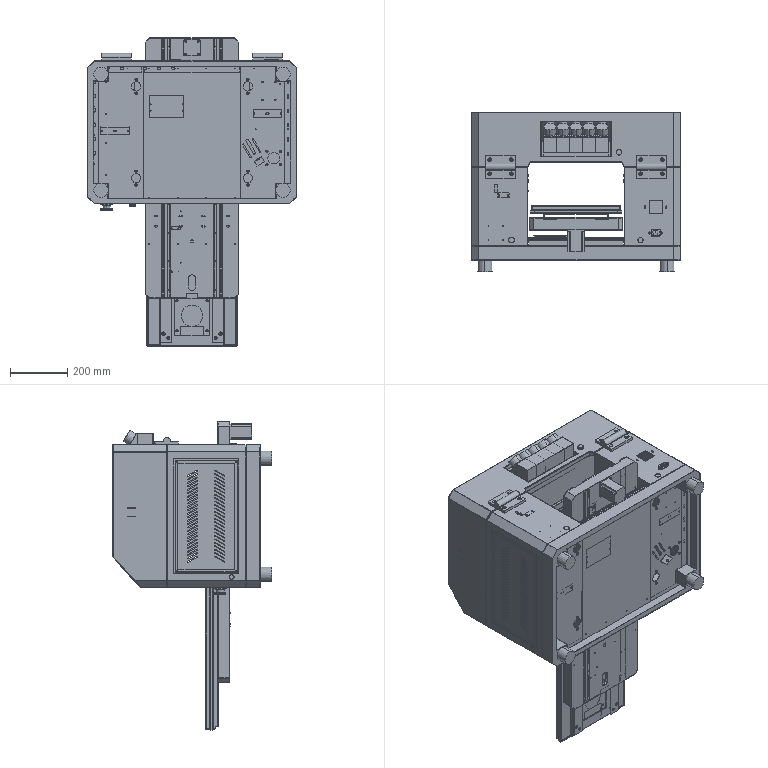Part | SolidWorks | 111 solids | 8716 faces | volume 12080386 mm3 | cylinder 4733 | plane 2741 | spline 527 | sphere 340 | torus 212 | cone 163 | commonest cylinder face diameters 1.5 x764 3 x312 3.3 x270 2.5 x260 0.2 x239 6 x207